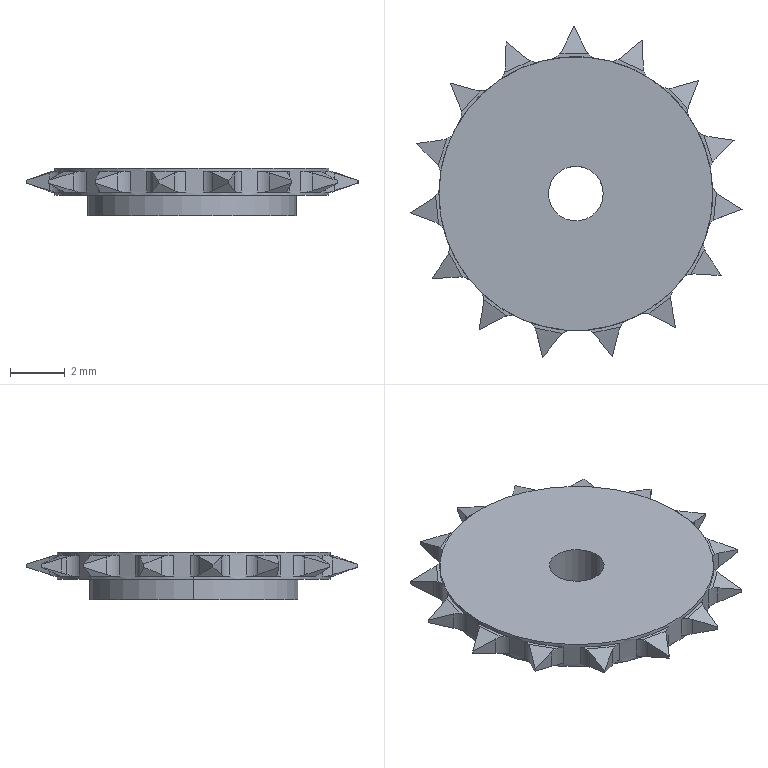Part | SolidWorks | features ICE 4, CirPattern 1, Extrusion 1 | 1 solid | 149 faces | box 12.129 x 12.076 x 1.75 mm | volume 112.986 mm3 | cylinder 101 | plane 48 | commonest cylinder face diameters 1.272 x34 50 x30 14.023 x16 17.771 x15 2 x2 7.624 x2